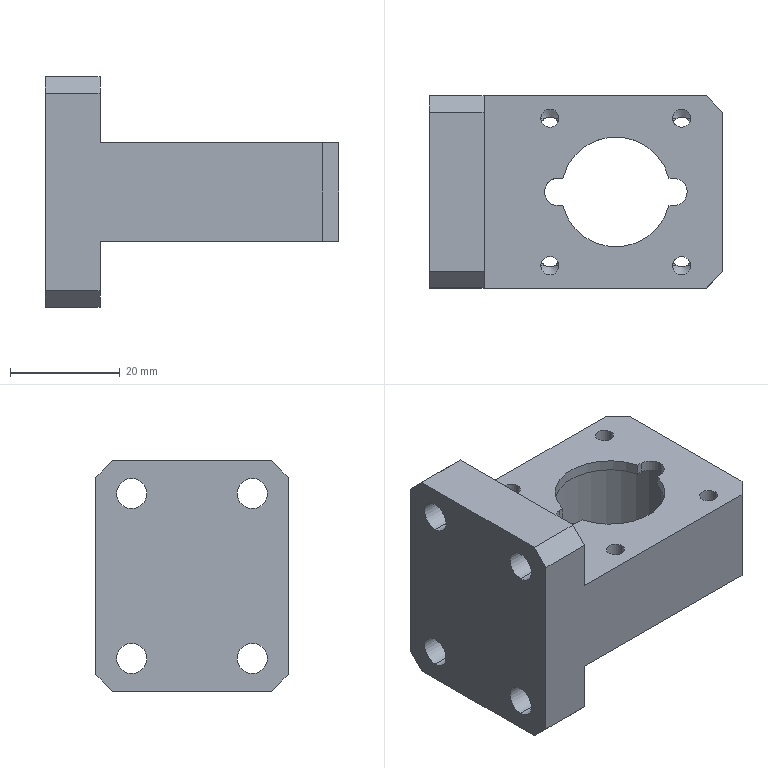Part | NX | features BREP 1 | 1 solid | 87 faces | box 53.5 x 35 x 42 mm | volume 30850 mm3 | cylinder 35 | cone 30 | plane 22 | commonest cylinder face diameters 3.3 x16 5.5 x8 2.5 x4 5 x3 20 x2 26 x2